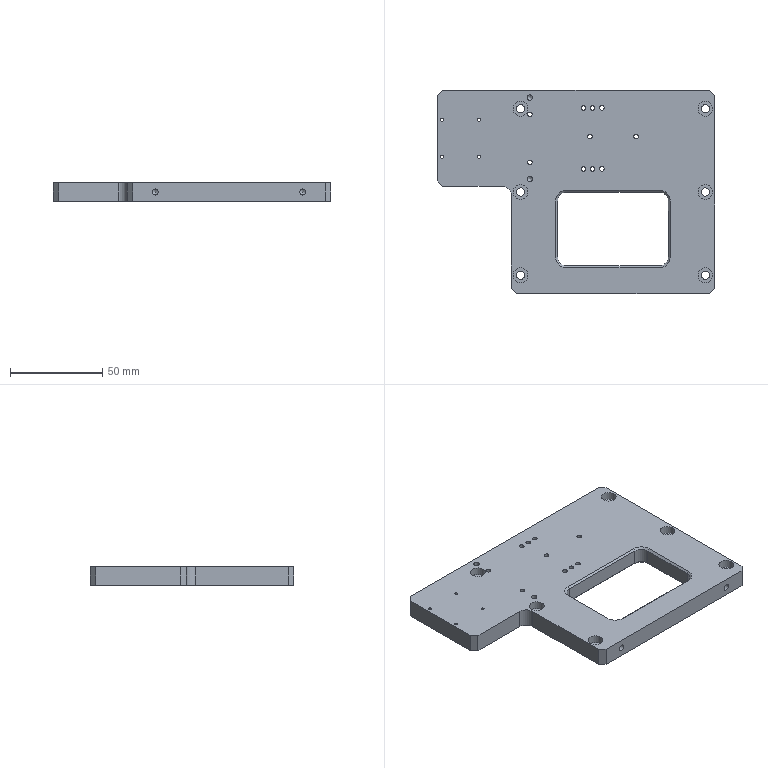Part | 1 solid | 78 faces | box 150 x 110 x 10 mm | volume 114978 mm3 | cylinder 35 | plane 31 | cone 12 | commonest cylinder face diameters 2.5 x10 4.5 x6 8 x6 10 x5 1.6 x4 3 x2